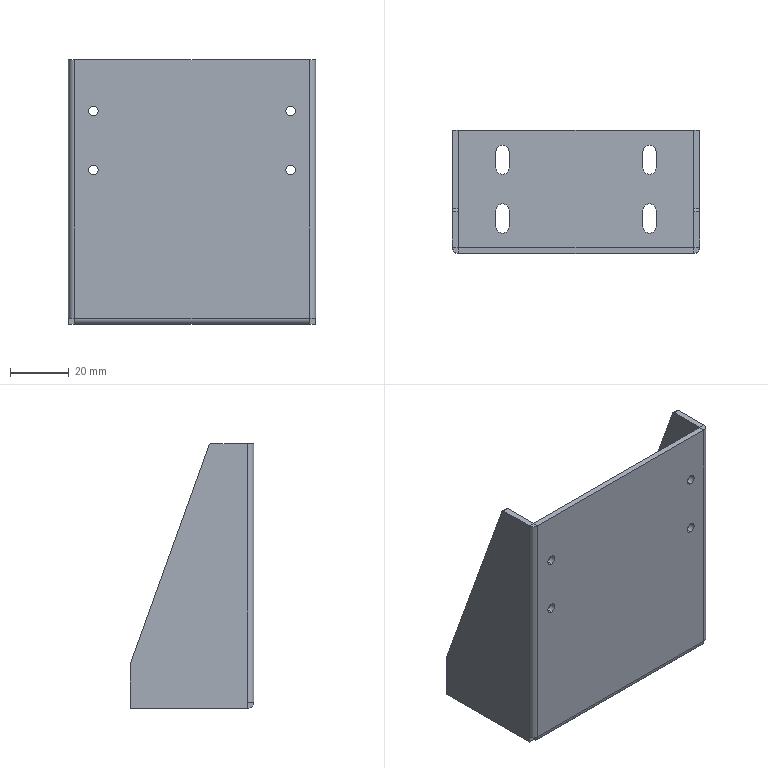Part | STEP file | 1 solid | 62 faces | box 84 x 42 x 90 mm | volume 31200 mm3 | plane 36 | cylinder 26 | commonest cylinder face diameters 3.3 x8 4.5 x8 2 x4 0.2 x3 4.2 x3